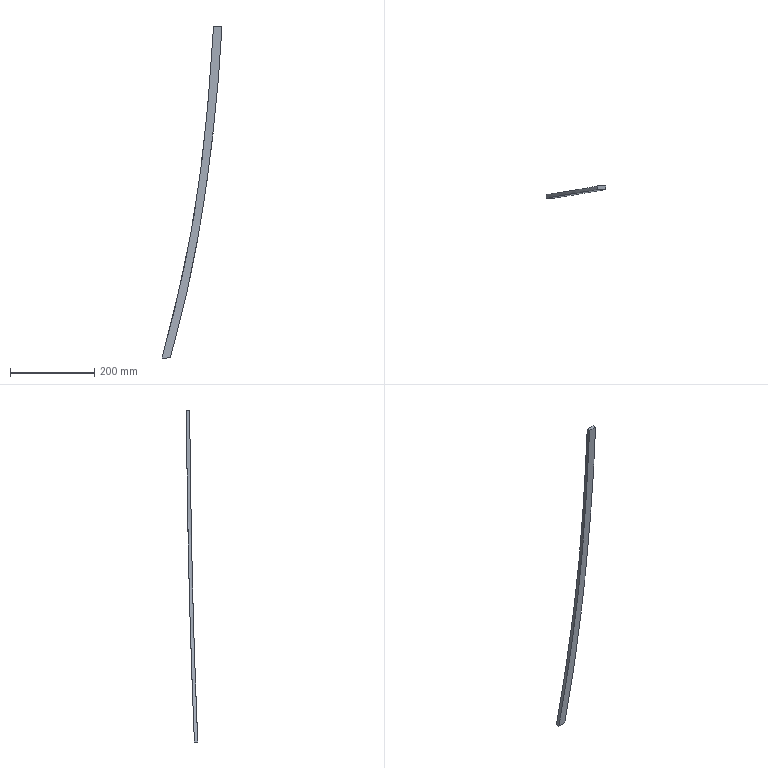Part | SolidWorks | features BaseBody 1 | 1 solid | 8 faces | box 142.386 x 27.255 x 788 mm | volume 121521 mm3 | spline 6 | plane 2